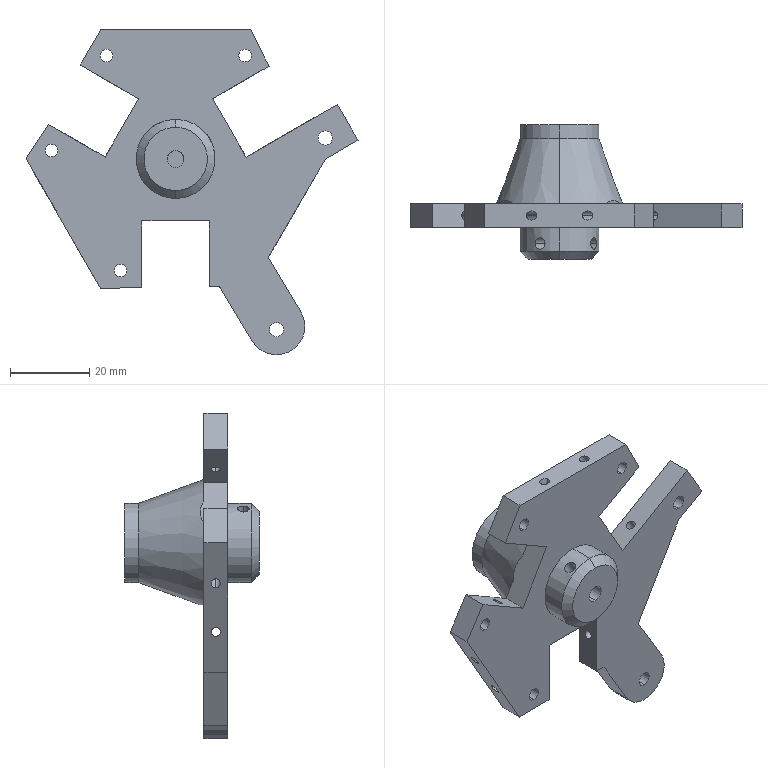Part | SolidWorks | features ICE 8, CirPattern 3, Chamfer 2, Cut 2, Extrusion 1 | 1 solid | 72 faces | box 83.855 x 34 x 82.22 mm | volume 30431 mm3 | cylinder 39 | plane 29 | cone 4 | commonest cylinder face diameters 2.3 x12 3.2 x8 2.9 x4 3.6 x4 4.2 x4 20 x4